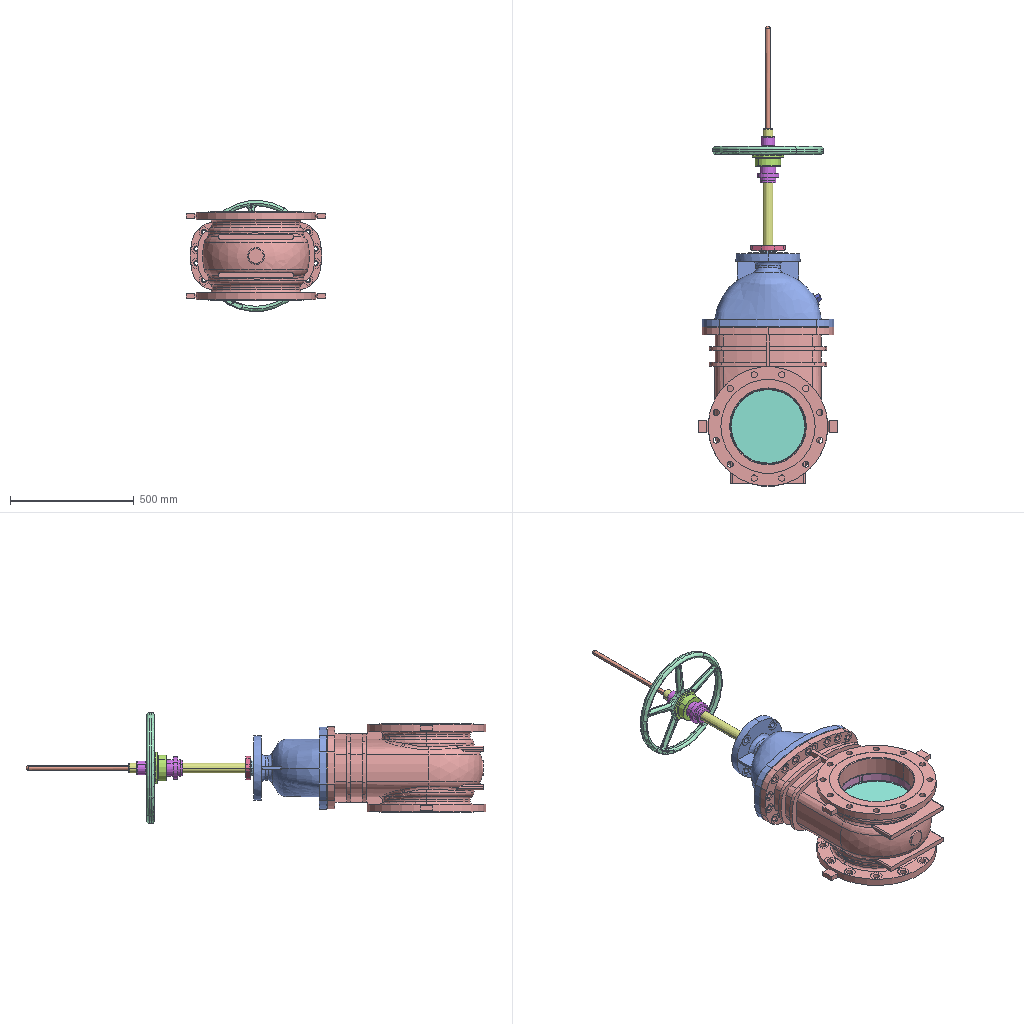Assembly | SolidWorks | 15 different items | 21 placed | box 563 x 1858 x 448 mm
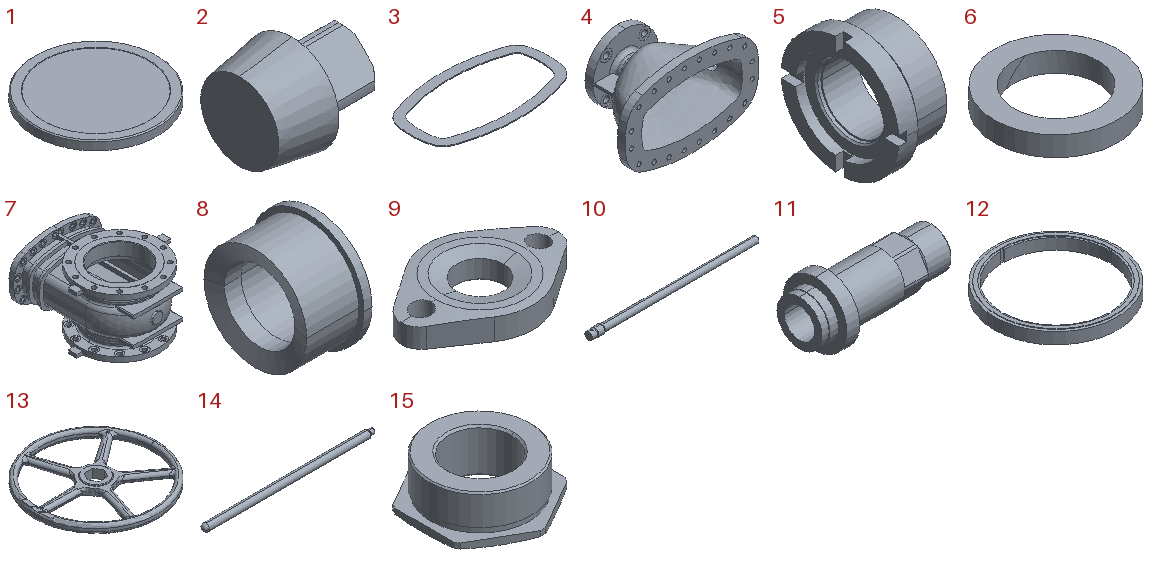Parts list (item | quantity | size | volume | features):
1 | x2 | 350 x 350 x 50 mm | 2420950 mm3 | features ICE 2, Chamfer 1, Extrusion 1, Fillet 1
2 | x1 | 40 x 36.354 x 36.354 mm | 26781 mm3 | features Chamfer 1, CirPattern 1, ICE 1, Revolution 1
3 | x1 | 460 x 260 x 3 mm | 101049 mm3 | features Extrusion 1
4 | x1 | 532 x 298 x 332 mm | 7097741 mm3 | features ICE 8, HoleWzd 4, Fillet 3, MirrorPattern 2, Blend 1, Chamfer 1, MoveFace 1, Revolution 1, Rib 1, Shell 1
5 | x1 | 35 x 74 x 74 mm | 68562 mm3 | features CirPattern 1, ICE 1, Revolution 1
6 | x5 | 59 x 59 x 9.5 mm | 14035 mm3 | features Extrusion 1, PLine 1
7 | x1 | 563 x 641.5 x 356 mm | 21607642 mm3 | features ICE 19, Fillet 7, MirrorPattern 4, MirrorSolid 4, Chamfer 3, CombineBodies 2, HoleWzd 2, Revolution 2, Split 2, Extrusion 1, MoveFace 1, RevCut 1, Rib 1, Sculpt 1
8 | x1 | 38 x 65 x 65 mm | 52156 mm3 | features ICE 3, Revolution 1
9 | x1 | 141 x 95 x 20 mm | 136049 mm3 | features Chamfer 1, Extrusion 1, RevCut 1
10 | x1 | 1010 x 50 x 50 mm | 1298621 mm3 | features Chamfer 2, HoleWzd 1, ICE 1, Revolution 1
11 | x1 | 186 x 89 x 89 mm | 390836 mm3 | features Chamfer 2, CirPattern 1, ICE 1, RevCut 1, Revolution 1
12 | x2 | 350 x 350 x 35 mm | 761867 mm3 | features ICE 6, CirPattern 1, Extrusion 1
13 | x1 | 450 x 450 x 32 mm | 1456731 mm3 | features ICE 5, Fillet 4, MoveFace 2, Blend 1, Chamfer 1, CirPattern 1, CombineBodies 1, Extrusion 1
14 | x1 | 430 x 18 x 18 mm | 106301 mm3 | features Chamfer 1, Revolution 1
15 | x1 | 115 x 130 x 45 mm | 256191 mm3 | features ICE 4, Chamfer 2, Extrusion 1
Mates (type | each side: item.copy, entity, surface, feature):
Concentric | 7.1 face cylinder Boss-Extrude8 | 4.1 face cylinder Boss-Extrude5 | 2 times
Concentric | 7.1 face cylinder Cut-Extrude4 | 12.1 face cylinder Cut-Extrude4
Coincident | 7.1 face plane Cut-Extrude4 | 12.1 face plane Boss-Extrude1
Concentric | 7.1 face cylinder Cut-Extrude3 | 1.1 face cylinder Boss-Extrude1
Coincident | 12.1 face plane Boss-Extrude1 | 1.1 face plane Boss-Extrude1
Concentric | 7.1 face cylinder Boss-Extrude8 | 3.1 face cylinder Boss-Extrude1 | 2 times
Concentric | assembly face | assembly face | 11 times
Concentric | 4.1 face cylinder CBORE for M16 Hex Head Bolt2 | assembly face
Coincident | 4.1 face plane CBORE for M16 Hex Head Bolt2 | assembly face
Coincident | 7.1 face plane Boss-Extrude7 | 3.1 face plane Boss-Extrude1
Coincident | 4.1 face plane Loft1 | 3.1 face plane Boss-Extrude1
Coincident | 7.1 face plane CBORE for M45 Hex Head Bolt2 | assembly face
Concentric | 4.1 face cylinder Cut-Extrude2 | 5.1 face cylinder Revolve1
Coincident | 4.1 face plane Cut-Extrude1 | 5.1 face plane Revolve1
Concentric | 4.1 face cylinder Cut-Extrude4 | 6.1 face cylinder Split Line1
Coincident | 5.1 face plane Revolve1 | 6.1 face plane Boss-Extrude1
Concentric | 4.1 face cylinder CBORE for M16 Hex Head Bolt1 | assembly face
Concentric | 4.1 face cylinder Cut-Extrude4 | 9.1 face cylinder Cut-Revolve1
Concentric | 4.1 face cylinder Cut-Extrude4 | 8.1 face cylinder Revolve1
Tangent | 9.1 face cone Cut-Revolve1 | 8.1 face sphere Revolve1
Concentric | 6.2 face cylinder Split Line1 | 6.3 face cylinder Split Line1
Concentric | 6.2 face cylinder Split Line1 | 6.4 face cylinder Split Line1
Concentric | 6.4 face cylinder Split Line1 | 6.5 face cylinder Split Line1
Coincident | 6.4 face plane Boss-Extrude1 | 6.5 face plane Boss-Extrude1
Coincident | 6.2 face plane Boss-Extrude1 | 6.4 face plane Boss-Extrude1
Coincident | 6.2 face plane Boss-Extrude1 | 6.3 face plane Boss-Extrude1
Concentric | 4.1 face cylinder Cut-Extrude4 | 6.5 face cylinder Split Line1
Coincident | 6.1 face plane Boss-Extrude1 | 6.3 face plane Boss-Extrude1
Coincident | 8.1 edge | 6.5 face plane Boss-Extrude1
Concentric | 9.1 face cylinder Boss-Extrude1 | assembly face
Concentric | 4.1 face cylinder M16 Tapped Hole1 | assembly face
Coincident | 4.1 edge | assembly face
Coincident | 9.1 face plane Boss-Extrude1 | assembly face
Concentric | 9.1 face cylinder Cut-Revolve1 | 10.1 face cylinder Revolve1
Concentric | 4.1 face cylinder Boss-Extrude3 | assembly face
Coincident | 4.1 face plane Boss-Extrude3 | assembly face
Coincident | assembly face | assembly face | 8 times
Coincident | 4.1 face plane CBORE for M16 Hex Head Bolt1 | assembly face
DistanceDim | assembly face | assembly face
Concentric | assembly face | 11.1 face cylinder Revolve1
Concentric | 11.1 face cylinder Revolve1 | assembly face
Coincident | 11.1 face plane Revolve1 | assembly face | 2 times
Concentric | 15.1 face cylinder Boss-Extrude2 | assembly face
Coincident | 15.1 face plane Boss-Extrude1 | assembly face
Concentric | 10.1 face cylinder Revolve1 | 13.1 face cylinder Boss-Extrude3
Parallel | 11.1 face plane Cut-Extrude1 | 13.1 face plane Cut-Extrude2
Coincident | 11.1 face plane CirPattern1 | 13.1 face plane Boss-Extrude2
Concentric | 10.1 face cylinder Revolve1 | assembly face | 2 times
Concentric | assembly face | 14.1 face cylinder Revolve2
Coincident | 10.1 face plane Revolve1 | 14.1 face plane Revolve2
Tangent | assembly face | assembly face
Concentric | 4.1 face cylinder M45 Tapped Hole1 | 2.1 face cone Revolve1
Coincident | 4.1 face plane Revolve1 | 2.1 face plane Revolve1
Concentric | 10.1 face cylinder Cut-Extrude1 | assembly face | 2 times
Concentric | 1.1 face cylinder Boss-Extrude1 | assembly face
Coincident | 1.1 face plane Boss-Extrude2 | assembly face
Concentric | 7.1 face cylinder Mirror9 | 12.2 face cylinder Boss-Extrude1
Coincident | 7.1 face plane Mirror9 | 12.2 face plane Boss-Extrude1
Concentric | 12.2 face cylinder Cut-Extrude4 | 1.2 face cylinder Boss-Extrude1
Coincident | 12.2 face plane Boss-Extrude1 | 1.2 face plane Boss-Extrude1
Parallel | assembly face | assembly face